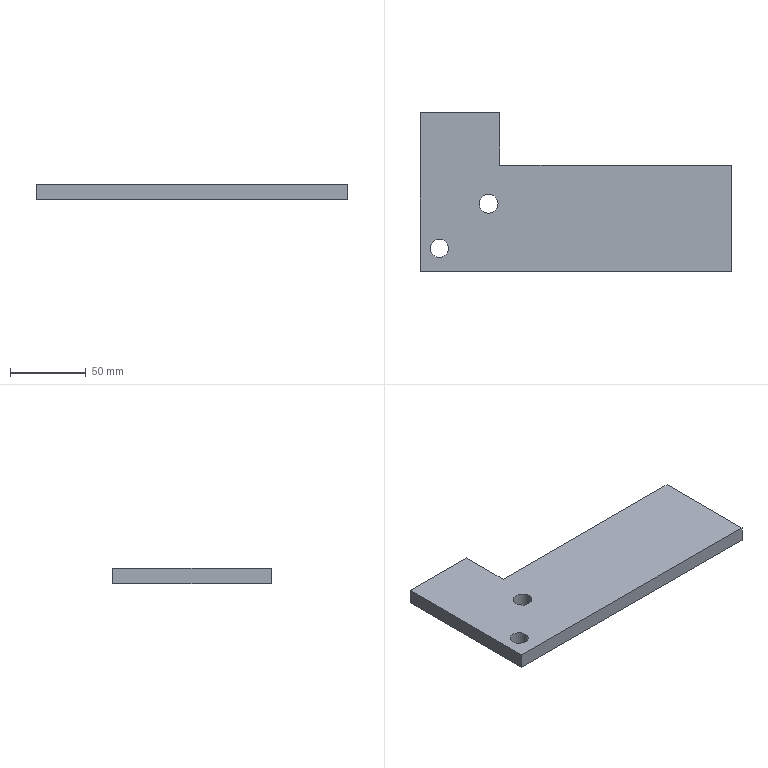Part | SolidWorks | features Extrusion 1 | 1 solid | 12 faces | box 205.392 x 104.5 x 10 mm | volume 159512 mm3 | plane 8 | cylinder 4 | commonest cylinder face diameters 12 x2 12.5 x2
STEP:
#1=CARTESIAN_POINT('',(46.3,-25.5,10.));
#2=VERTEX_POINT('',#1);
#3=CARTESIAN_POINT('',(58.8,-25.5,10.));
#4=VERTEX_POINT('',#3);
#5=CARTESIAN_POINT('',(52.55,-25.5,10.));
#6=DIRECTION('',(0.,0.,1.));
#7=DIRECTION('',(1.,0.,0.));
#8=AXIS2_PLACEMENT_3D('',#5,#6,#7);
#9=CIRCLE('',#8,6.25);
#10=EDGE_CURVE('',#2,#4,#9,.T.);
#11=ORIENTED_EDGE('',*,*,#10,.T.);
#12=CARTESIAN_POINT('',(58.8,-25.5,0.));
#13=VERTEX_POINT('',#12);
#14=CARTESIAN_POINT('',(58.8,-25.5,10.));
#15=DIRECTION('',(0.,0.,-1.));
#16=VECTOR('',#15,1000.);
#17=LINE('',#14,#16);
#18=EDGE_CURVE('',#4,#13,#17,.T.);
#19=ORIENTED_EDGE('',*,*,#18,.T.);
#20=CARTESIAN_POINT('',(46.3,-25.5,0.));
#21=VERTEX_POINT('',#20);
#22=CARTESIAN_POINT('',(52.55,-25.5,0.));
#23=DIRECTION('',(0.,0.,1.));
#24=DIRECTION('',(1.,0.,0.));
#25=AXIS2_PLACEMENT_3D('',#22,#23,#24);
#26=CIRCLE('',#25,6.25);
#27=EDGE_CURVE('',#21,#13,#26,.T.);
#28=ORIENTED_EDGE('',*,*,#27,.F.);
#29=CARTESIAN_POINT('',(46.3,-25.5,10.));
#30=DIRECTION('',(0.,0.,-1.));
#31=VECTOR('',#30,1000.);
#32=LINE('',#29,#31);
#33=EDGE_CURVE('',#2,#21,#32,.T.);
#34=ORIENTED_EDGE('',*,*,#33,.F.);
#35=EDGE_LOOP('',(#11,#19,#28,#34));
#36=FACE_OUTER_BOUND('',#35,.T.);
#37=CARTESIAN_POINT('',(52.55,-25.5,10.));
#38=DIRECTION('',(0.,0.,-1.));
#39=DIRECTION('',(-1.,0.,0.));
#40=AXIS2_PLACEMENT_3D('',#37,#38,#39);
#41=CYLINDRICAL_SURFACE('',#40,6.25);
#42=ADVANCED_FACE('',(#36),#41,.F.);
#43=CARTESIAN_POINT('',(14.,-55.,10.));
#44=VERTEX_POINT('',#43);
#45=CARTESIAN_POINT('',(26.,-55.,10.));
#46=VERTEX_POINT('',#45);
#47=CARTESIAN_POINT('',(20.,-55.,10.));
#48=DIRECTION('',(0.,0.,1.));
#49=DIRECTION('',(1.,0.,0.));
#50=AXIS2_PLACEMENT_3D('',#47,#48,#49);
#51=CIRCLE('',#50,6.);
#52=EDGE_CURVE('',#44,#46,#51,.T.);
#53=ORIENTED_EDGE('',*,*,#52,.T.);
#54=CARTESIAN_POINT('',(26.,-55.,0.));
#55=VERTEX_POINT('',#54);
#56=CARTESIAN_POINT('',(26.,-55.,10.));
#57=DIRECTION('',(0.,0.,-1.));
#58=VECTOR('',#57,1000.);
#59=LINE('',#56,#58);
#60=EDGE_CURVE('',#46,#55,#59,.T.);
#61=ORIENTED_EDGE('',*,*,#60,.T.);
#62=CARTESIAN_POINT('',(14.,-55.,0.));
#63=VERTEX_POINT('',#62);
#64=CARTESIAN_POINT('',(20.,-55.,0.));
#65=DIRECTION('',(0.,0.,1.));
#66=DIRECTION('',(1.,0.,0.));
#67=AXIS2_PLACEMENT_3D('',#64,#65,#66);
#68=CIRCLE('',#67,6.);
#69=EDGE_CURVE('',#63,#55,#68,.T.);
#70=ORIENTED_EDGE('',*,*,#69,.F.);
#71=CARTESIAN_POINT('',(14.,-55.,10.));
#72=DIRECTION('',(0.,0.,-1.));
#73=VECTOR('',#72,1000.);
#74=LINE('',#71,#73);
#75=EDGE_CURVE('',#44,#63,#74,.T.);
#76=ORIENTED_EDGE('',*,*,#75,.F.);
#77=EDGE_LOOP('',(#53,#61,#70,#76));
#78=FACE_OUTER_BOUND('',#77,.T.);
#79=CARTESIAN_POINT('',(20.,-55.,10.));
#80=DIRECTION('',(0.,0.,-1.));
#81=DIRECTION('',(-1.,0.,0.));
#82=AXIS2_PLACEMENT_3D('',#79,#80,#81);
#83=CYLINDRICAL_SURFACE('',#82,6.);
#84=ADVANCED_FACE('',(#78),#83,.F.);
#85=ORIENTED_EDGE('',*,*,#52,.F.);
#86=CARTESIAN_POINT('',(20.,-55.,10.));
#87=DIRECTION('',(0.,0.,1.));
#88=DIRECTION('',(1.,0.,0.));
#89=AXIS2_PLACEMENT_3D('',#86,#87,#88);
#90=CIRCLE('',#89,6.);
#91=EDGE_CURVE('',#46,#44,#90,.T.);
#92=ORIENTED_EDGE('',*,*,#91,.F.);
#93=EDGE_LOOP('',(#85,#92));
#94=FACE_BOUND('',#93,.T.);
#95=CARTESIAN_POINT('',(212.942,-70.,10.));
#96=VERTEX_POINT('',#95);
#97=CARTESIAN_POINT('',(212.942,0.,10.));
#98=VERTEX_POINT('',#97);
#99=CARTESIAN_POINT('',(212.942,-70.,10.));
#100=DIRECTION('',(0.,1.,0.));
#101=VECTOR('',#100,1000.);
#102=LINE('',#99,#101);
#103=EDGE_CURVE('',#96,#98,#102,.T.);
#104=ORIENTED_EDGE('',*,*,#103,.T.);
#105=CARTESIAN_POINT('',(60.,0.,10.));
#106=VERTEX_POINT('',#105);
#107=CARTESIAN_POINT('',(212.942,0.,10.));
#108=DIRECTION('',(-1.,0.,0.));
#109=VECTOR('',#108,1000.);
#110=LINE('',#107,#109);
#111=EDGE_CURVE('',#98,#106,#110,.T.);
#112=ORIENTED_EDGE('',*,*,#111,.T.);
#113=CARTESIAN_POINT('',(60.,34.5,10.));
#114=VERTEX_POINT('',#113);
#115=CARTESIAN_POINT('',(60.,34.5,10.));
#116=DIRECTION('',(0.,1.,0.));
#117=VECTOR('',#116,1000.);
#118=LINE('',#115,#117);
#119=EDGE_CURVE('',#106,#114,#118,.T.);
#120=ORIENTED_EDGE('',*,*,#119,.T.);
#121=CARTESIAN_POINT('',(7.55,34.5,10.));
#122=VERTEX_POINT('',#121);
#123=CARTESIAN_POINT('',(60.,34.5,10.));
#124=DIRECTION('',(-1.,0.,0.));
#125=VECTOR('',#124,1000.);
#126=LINE('',#123,#125);
#127=EDGE_CURVE('',#114,#122,#126,.T.);
#128=ORIENTED_EDGE('',*,*,#127,.T.);
#129=CARTESIAN_POINT('',(7.55,-70.,10.));
#130=VERTEX_POINT('',#129);
#131=CARTESIAN_POINT('',(7.55,34.5,10.));
#132=DIRECTION('',(0.,-1.,0.));
#133=VECTOR('',#132,1000.);
#134=LINE('',#131,#133);
#135=EDGE_CURVE('',#122,#130,#134,.T.);
#136=ORIENTED_EDGE('',*,*,#135,.T.);
#137=CARTESIAN_POINT('',(7.55,-70.,10.));
#138=DIRECTION('',(1.,0.,0.));
#139=VECTOR('',#138,1000.);
#140=LINE('',#137,#139);
#141=EDGE_CURVE('',#130,#96,#140,.T.);
#142=ORIENTED_EDGE('',*,*,#141,.T.);
#143=EDGE_LOOP('',(#104,#112,#120,#128,#136,#142));
#144=FACE_OUTER_BOUND('',#143,.T.);
#145=ORIENTED_EDGE('',*,*,#10,.F.);
#146=CARTESIAN_POINT('',(52.55,-25.5,10.));
#147=DIRECTION('',(0.,0.,1.));
#148=DIRECTION('',(1.,0.,0.));
#149=AXIS2_PLACEMENT_3D('',#146,#147,#148);
#150=CIRCLE('',#149,6.25);
#151=EDGE_CURVE('',#4,#2,#150,.T.);
#152=ORIENTED_EDGE('',*,*,#151,.F.);
#153=EDGE_LOOP('',(#145,#152));
#154=FACE_BOUND('',#153,.T.);
#155=CARTESIAN_POINT('',(0.,0.,10.));
#156=DIRECTION('',(0.,0.,1.));
#157=DIRECTION('',(1.,0.,0.));
#158=AXIS2_PLACEMENT_3D('',#155,#156,#157);
#159=PLANE('',#158);
#160=ADVANCED_FACE('',(#94,#144,#154),#159,.T.);
#161=CARTESIAN_POINT('',(212.942,-70.,0.));
#162=VERTEX_POINT('',#161);
#163=CARTESIAN_POINT('',(212.942,0.,0.));
#164=VERTEX_POINT('',#163);
#165=CARTESIAN_POINT('',(212.942,-70.,0.));
#166=DIRECTION('',(0.,1.,0.));
#167=VECTOR('',#166,1000.);
#168=LINE('',#165,#167);
#169=EDGE_CURVE('',#162,#164,#168,.T.);
#170=ORIENTED_EDGE('',*,*,#169,.F.);
#171=CARTESIAN_POINT('',(7.55,-70.,0.));
#172=VERTEX_POINT('',#171);
#173=CARTESIAN_POINT('',(7.55,-70.,0.));
#174=DIRECTION('',(1.,0.,0.));
#175=VECTOR('',#174,1000.);
#176=LINE('',#173,#175);
#177=EDGE_CURVE('',#172,#162,#176,.T.);
#178=ORIENTED_EDGE('',*,*,#177,.F.);
#179=CARTESIAN_POINT('',(7.55,34.5,0.));
#180=VERTEX_POINT('',#179);
#181=CARTESIAN_POINT('',(7.55,34.5,0.));
#182=DIRECTION('',(0.,-1.,0.));
#183=VECTOR('',#182,1000.);
#184=LINE('',#181,#183);
#185=EDGE_CURVE('',#180,#172,#184,.T.);
#186=ORIENTED_EDGE('',*,*,#185,.F.);
#187=CARTESIAN_POINT('',(60.,34.5,0.));
#188=VERTEX_POINT('',#187);
#189=CARTESIAN_POINT('',(60.,34.5,0.));
#190=DIRECTION('',(-1.,0.,0.));
#191=VECTOR('',#190,1000.);
#192=LINE('',#189,#191);
#193=EDGE_CURVE('',#188,#180,#192,.T.);
#194=ORIENTED_EDGE('',*,*,#193,.F.);
#195=CARTESIAN_POINT('',(60.,0.,0.));
#196=VERTEX_POINT('',#195);
#197=CARTESIAN_POINT('',(60.,34.5,0.));
#198=DIRECTION('',(0.,1.,0.));
#199=VECTOR('',#198,1000.);
#200=LINE('',#197,#199);
#201=EDGE_CURVE('',#196,#188,#200,.T.);
#202=ORIENTED_EDGE('',*,*,#201,.F.);
#203=CARTESIAN_POINT('',(60.,0.,0.));
#204=DIRECTION('',(-1.,0.,0.));
#205=VECTOR('',#204,1000.);
#206=LINE('',#203,#205);
#207=EDGE_CURVE('',#164,#196,#206,.T.);
#208=ORIENTED_EDGE('',*,*,#207,.F.);
#209=EDGE_LOOP('',(#170,#178,#186,#194,#202,#208));
#210=FACE_OUTER_BOUND('',#209,.T.);
#211=ORIENTED_EDGE('',*,*,#69,.T.);
#212=CARTESIAN_POINT('',(20.,-55.,0.));
#213=DIRECTION('',(0.,0.,1.));
#214=DIRECTION('',(1.,0.,0.));
#215=AXIS2_PLACEMENT_3D('',#212,#213,#214);
#216=CIRCLE('',#215,6.);
#217=EDGE_CURVE('',#55,#63,#216,.T.);
#218=ORIENTED_EDGE('',*,*,#217,.T.);
#219=EDGE_LOOP('',(#211,#218));
#220=FACE_BOUND('',#219,.T.);
#221=ORIENTED_EDGE('',*,*,#27,.T.);
#222=CARTESIAN_POINT('',(52.55,-25.5,0.));
#223=DIRECTION('',(0.,0.,1.));
#224=DIRECTION('',(1.,0.,0.));
#225=AXIS2_PLACEMENT_3D('',#222,#223,#224);
#226=CIRCLE('',#225,6.25);
#227=EDGE_CURVE('',#13,#21,#226,.T.);
#228=ORIENTED_EDGE('',*,*,#227,.T.);
#229=EDGE_LOOP('',(#221,#228));
#230=FACE_BOUND('',#229,.T.);
#231=CARTESIAN_POINT('',(0.,0.,0.));
#232=DIRECTION('',(0.,0.,1.));
#233=DIRECTION('',(1.,0.,0.));
#234=AXIS2_PLACEMENT_3D('',#231,#232,#233);
#235=PLANE('',#234);
#236=ADVANCED_FACE('',(#210,#220,#230),#235,.F.);
#237=ORIENTED_EDGE('',*,*,#169,.T.);
#238=CARTESIAN_POINT('',(212.942,0.,10.));
#239=DIRECTION('',(0.,0.,-1.));
#240=VECTOR('',#239,1000.);
#241=LINE('',#238,#240);
#242=EDGE_CURVE('',#98,#164,#241,.T.);
#243=ORIENTED_EDGE('',*,*,#242,.F.);
#244=ORIENTED_EDGE('',*,*,#103,.F.);
#245=CARTESIAN_POINT('',(212.942,-70.,10.));
#246=DIRECTION('',(0.,0.,-1.));
#247=VECTOR('',#246,1000.);
#248=LINE('',#245,#247);
#249=EDGE_CURVE('',#96,#162,#248,.T.);
#250=ORIENTED_EDGE('',*,*,#249,.T.);
#251=EDGE_LOOP('',(#237,#243,#244,#250));
#252=FACE_OUTER_BOUND('',#251,.T.);
#253=CARTESIAN_POINT('',(212.942,-70.,10.));
#254=DIRECTION('',(-1.,0.,0.));
#255=DIRECTION('',(0.,0.,1.));
#256=AXIS2_PLACEMENT_3D('',#253,#254,#255);
#257=PLANE('',#256);
#258=ADVANCED_FACE('',(#252),#257,.F.);
#259=ORIENTED_EDGE('',*,*,#207,.T.);
#260=CARTESIAN_POINT('',(60.,0.,10.));
#261=DIRECTION('',(0.,0.,-1.));
#262=VECTOR('',#261,1000.);
#263=LINE('',#260,#262);
#264=EDGE_CURVE('',#106,#196,#263,.T.);
#265=ORIENTED_EDGE('',*,*,#264,.F.);
#266=ORIENTED_EDGE('',*,*,#111,.F.);
#267=ORIENTED_EDGE('',*,*,#242,.T.);
#268=EDGE_LOOP('',(#259,#265,#266,#267));
#269=FACE_OUTER_BOUND('',#268,.T.);
#270=CARTESIAN_POINT('',(60.,0.,10.));
#271=DIRECTION('',(0.,-1.,0.));
#272=DIRECTION('',(1.,0.,0.));
#273=AXIS2_PLACEMENT_3D('',#270,#271,#272);
#274=PLANE('',#273);
#275=ADVANCED_FACE('',(#269),#274,.F.);
#276=ORIENTED_EDGE('',*,*,#201,.T.);
#277=CARTESIAN_POINT('',(60.,34.5,10.));
#278=DIRECTION('',(0.,0.,-1.));
#279=VECTOR('',#278,1000.);
#280=LINE('',#277,#279);
#281=EDGE_CURVE('',#114,#188,#280,.T.);
#282=ORIENTED_EDGE('',*,*,#281,.F.);
#283=ORIENTED_EDGE('',*,*,#119,.F.);
#284=ORIENTED_EDGE('',*,*,#264,.T.);
#285=EDGE_LOOP('',(#276,#282,#283,#284));
#286=FACE_OUTER_BOUND('',#285,.T.);
#287=CARTESIAN_POINT('',(60.,34.5,10.));
#288=DIRECTION('',(-1.,0.,0.));
#289=DIRECTION('',(0.,-1.,0.));
#290=AXIS2_PLACEMENT_3D('',#287,#288,#289);
#291=PLANE('',#290);
#292=ADVANCED_FACE('',(#286),#291,.F.);
#293=ORIENTED_EDGE('',*,*,#193,.T.);
#294=CARTESIAN_POINT('',(7.55,34.5,10.));
#295=DIRECTION('',(0.,0.,-1.));
#296=VECTOR('',#295,1000.);
#297=LINE('',#294,#296);
#298=EDGE_CURVE('',#122,#180,#297,.T.);
#299=ORIENTED_EDGE('',*,*,#298,.F.);
#300=ORIENTED_EDGE('',*,*,#127,.F.);
#301=ORIENTED_EDGE('',*,*,#281,.T.);
#302=EDGE_LOOP('',(#293,#299,#300,#301));
#303=FACE_OUTER_BOUND('',#302,.T.);
#304=CARTESIAN_POINT('',(60.,34.5,10.));
#305=DIRECTION('',(0.,-1.,0.));
#306=DIRECTION('',(0.,0.,-1.));
#307=AXIS2_PLACEMENT_3D('',#304,#305,#306);
#308=PLANE('',#307);
#309=ADVANCED_FACE('',(#303),#308,.F.);
#310=ORIENTED_EDGE('',*,*,#185,.T.);
#311=CARTESIAN_POINT('',(7.55,-70.,10.));
#312=DIRECTION('',(0.,0.,-1.));
#313=VECTOR('',#312,1000.);
#314=LINE('',#311,#313);
#315=EDGE_CURVE('',#130,#172,#314,.T.);
#316=ORIENTED_EDGE('',*,*,#315,.F.);
#317=ORIENTED_EDGE('',*,*,#135,.F.);
#318=ORIENTED_EDGE('',*,*,#298,.T.);
#319=EDGE_LOOP('',(#310,#316,#317,#318));
#320=FACE_OUTER_BOUND('',#319,.T.);
#321=CARTESIAN_POINT('',(7.55,34.5,10.));
#322=DIRECTION('',(1.,0.,0.));
#323=DIRECTION('',(0.,1.,0.));
#324=AXIS2_PLACEMENT_3D('',#321,#322,#323);
#325=PLANE('',#324);
#326=ADVANCED_FACE('',(#320),#325,.F.);
#327=ORIENTED_EDGE('',*,*,#177,.T.);
#328=ORIENTED_EDGE('',*,*,#249,.F.);
#329=ORIENTED_EDGE('',*,*,#141,.F.);
#330=ORIENTED_EDGE('',*,*,#315,.T.);
#331=EDGE_LOOP('',(#327,#328,#329,#330));
#332=FACE_OUTER_BOUND('',#331,.T.);
#333=CARTESIAN_POINT('',(7.55,-70.,10.));
#334=DIRECTION('',(0.,1.,0.));
#335=DIRECTION('',(0.,0.,1.));
#336=AXIS2_PLACEMENT_3D('',#333,#334,#335);
#337=PLANE('',#336);
#338=ADVANCED_FACE('',(#332),#337,.F.);
#339=ORIENTED_EDGE('',*,*,#60,.F.);
#340=ORIENTED_EDGE('',*,*,#91,.T.);
#341=ORIENTED_EDGE('',*,*,#75,.T.);
#342=ORIENTED_EDGE('',*,*,#217,.F.);
#343=EDGE_LOOP('',(#339,#340,#341,#342));
#344=FACE_OUTER_BOUND('',#343,.T.);
#345=CARTESIAN_POINT('',(20.,-55.,10.));
#346=DIRECTION('',(0.,0.,-1.));
#347=DIRECTION('',(-1.,0.,0.));
#348=AXIS2_PLACEMENT_3D('',#345,#346,#347);
#349=CYLINDRICAL_SURFACE('',#348,6.);
#350=ADVANCED_FACE('',(#344),#349,.F.);
#351=ORIENTED_EDGE('',*,*,#18,.F.);
#352=ORIENTED_EDGE('',*,*,#151,.T.);
#353=ORIENTED_EDGE('',*,*,#33,.T.);
#354=ORIENTED_EDGE('',*,*,#227,.F.);
#355=EDGE_LOOP('',(#351,#352,#353,#354));
#356=FACE_OUTER_BOUND('',#355,.T.);
#357=CARTESIAN_POINT('',(52.55,-25.5,10.));
#358=DIRECTION('',(0.,0.,-1.));
#359=DIRECTION('',(-1.,0.,0.));
#360=AXIS2_PLACEMENT_3D('',#357,#358,#359);
#361=CYLINDRICAL_SURFACE('',#360,6.25);
#362=ADVANCED_FACE('',(#356),#361,.F.);
#363=CLOSED_SHELL('',(#42,#84,#160,#236,#258,#275,#292,#309,#326,#338,#350,#362));
#364=MANIFOLD_SOLID_BREP('',#363);
#365=CARTESIAN_POINT('',(0.,0.,0.));
#366=DIRECTION('',(0.,0.,1.));
#367=DIRECTION('',(1.,0.,0.));
#368=AXIS2_PLACEMENT_3D('',#365,#366,#367);
#369=(LENGTH_UNIT()NAMED_UNIT(*)SI_UNIT(.MILLI.,.METRE.));
#370=UNCERTAINTY_MEASURE_WITH_UNIT(LENGTH_MEASURE(0.00001),#369,'','');
#371=(NAMED_UNIT(*)PLANE_ANGLE_UNIT()SI_UNIT($,.RADIAN.));
#372=(NAMED_UNIT(*)SI_UNIT($,.STERADIAN.)SOLID_ANGLE_UNIT());
#373=(GEOMETRIC_REPRESENTATION_CONTEXT(3)GLOBAL_UNCERTAINTY_ASSIGNED_CONTEXT((#370))GLOBAL_UNIT_ASSIGNED_CONTEXT((#369,#371,#372))REPRESENTATION_CONTEXT('',''));
#374=ADVANCED_BREP_SHAPE_REPRESENTATION('',(#364,#368),#373);